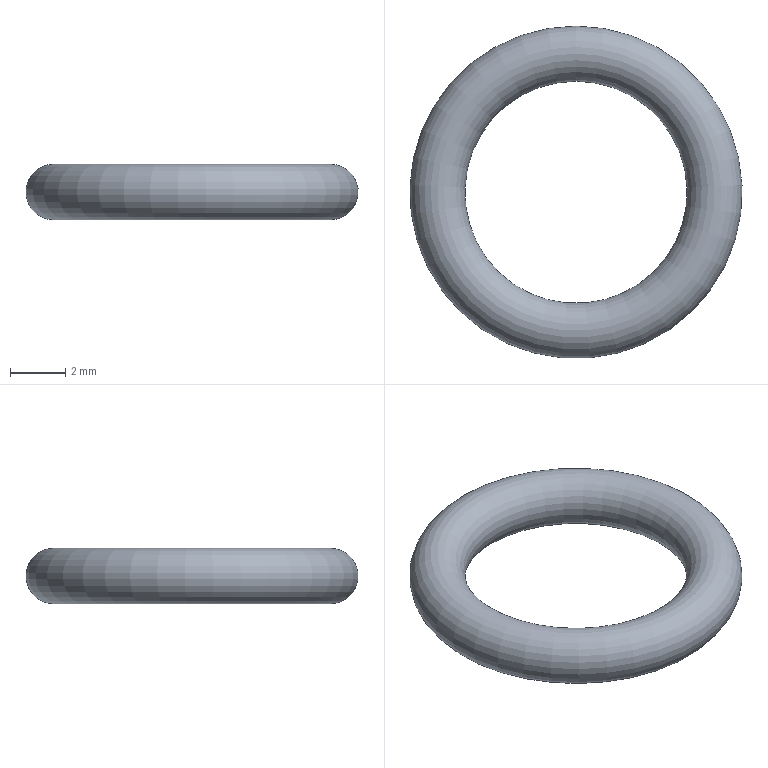Part | STEP file | 1-65.3 | 1 solid | 1 faces | box 12 x 12 x 2 mm | volume 98.696 mm3 | torus 1
STEP:
#1=CARTESIAN_POINT('',(0.,0.,0.));
#2=DIRECTION('',(0.,0.,1.));
#3=DIRECTION('',(1.,0.,0.));
#4=AXIS2_PLACEMENT_3D('',#1,#2,#3);
#5=CARTESIAN_POINT('',(0.,5.,-1.));
#6=VERTEX_POINT('',#5);
#7=CARTESIAN_POINT('',(0.,5.,0.));
#8=DIRECTION('',(-1.,0.,0.));
#9=DIRECTION('',(0.,0.,-1.));
#10=AXIS2_PLACEMENT_3D('',#7,#8,#9);
#11=CIRCLE('',#10,1.);
#12=CARTESIAN_POINT('',(0.,0.,0.));
#13=DIRECTION('',(0.,0.,-1.));
#14=DIRECTION('',(0.,1.,0.));
#15=AXIS2_PLACEMENT_3D('',#12,#13,#14);
#16=TOROIDAL_SURFACE('',#15,5.,1.);
#17=CARTESIAN_POINT('',(6.283,1.571));
#18=DIRECTION('',(0.,1.));
#19=VECTOR('',#18,1.);
#20=LINE('',#17,#19);
#21=(GEOMETRIC_REPRESENTATION_CONTEXT(2)PARAMETRIC_REPRESENTATION_CONTEXT()REPRESENTATION_CONTEXT('',''));
#22=DEFINITIONAL_REPRESENTATION('',(#20),#21);
#23=PCURVE('',#16,#22);
#24=CARTESIAN_POINT('',(0.,1.571));
#25=DIRECTION('',(0.,1.));
#26=VECTOR('',#25,1.);
#27=LINE('',#24,#26);
#28=(GEOMETRIC_REPRESENTATION_CONTEXT(2)PARAMETRIC_REPRESENTATION_CONTEXT()REPRESENTATION_CONTEXT('',''));
#29=DEFINITIONAL_REPRESENTATION('',(#27),#28);
#30=PCURVE('',#16,#29);
#31=SEAM_CURVE('',#11,(#23,#30),.PCURVE_S1.);
#32=EDGE_CURVE('',#6,#6,#31,.T.);
#33=ORIENTED_EDGE('',*,*,#32,.T.);
#34=CARTESIAN_POINT('',(0.,0.,-1.));
#35=DIRECTION('',(0.,0.,1.));
#36=DIRECTION('',(0.,1.,0.));
#37=AXIS2_PLACEMENT_3D('',#34,#35,#36);
#38=CIRCLE('',#37,5.);
#39=CARTESIAN_POINT('',(6.283,7.854));
#40=DIRECTION('',(-1.,0.));
#41=VECTOR('',#40,1.);
#42=LINE('',#39,#41);
#43=(GEOMETRIC_REPRESENTATION_CONTEXT(2)PARAMETRIC_REPRESENTATION_CONTEXT()REPRESENTATION_CONTEXT('',''));
#44=DEFINITIONAL_REPRESENTATION('',(#42),#43);
#45=PCURVE('',#16,#44);
#46=CARTESIAN_POINT('',(6.283,1.571));
#47=DIRECTION('',(-1.,0.));
#48=VECTOR('',#47,1.);
#49=LINE('',#46,#48);
#50=(GEOMETRIC_REPRESENTATION_CONTEXT(2)PARAMETRIC_REPRESENTATION_CONTEXT()REPRESENTATION_CONTEXT('',''));
#51=DEFINITIONAL_REPRESENTATION('',(#49),#50);
#52=PCURVE('',#16,#51);
#53=SEAM_CURVE('',#38,(#45,#52),.PCURVE_S1.);
#54=EDGE_CURVE('',#6,#6,#53,.T.);
#55=ORIENTED_EDGE('',*,*,#54,.T.);
#56=ORIENTED_EDGE('',*,*,#32,.F.);
#57=ORIENTED_EDGE('',*,*,#54,.F.);
#58=EDGE_LOOP('',(#33,#55,#56,#57));
#59=FACE_BOUND('',#58,.T.);
#60=ADVANCED_FACE('',(#59),#16,.T.);
#61=CLOSED_SHELL('',(#60));
#62=MANIFOLD_SOLID_BREP('',#61);
#63=(LENGTH_UNIT()NAMED_UNIT(*)SI_UNIT(.MILLI.,.METRE.));
#64=UNCERTAINTY_MEASURE_WITH_UNIT(LENGTH_MEASURE(0.0000001),#63,'','');
#65=(NAMED_UNIT(*)PLANE_ANGLE_UNIT()SI_UNIT($,.RADIAN.));
#66=(NAMED_UNIT(*)SI_UNIT($,.STERADIAN.)SOLID_ANGLE_UNIT());
#67=(GEOMETRIC_REPRESENTATION_CONTEXT(3)GLOBAL_UNCERTAINTY_ASSIGNED_CONTEXT((#64))GLOBAL_UNIT_ASSIGNED_CONTEXT((#63,#65,#66))REPRESENTATION_CONTEXT('',''));
#68=ADVANCED_BREP_SHAPE_REPRESENTATION('',(#4,#62),#67);